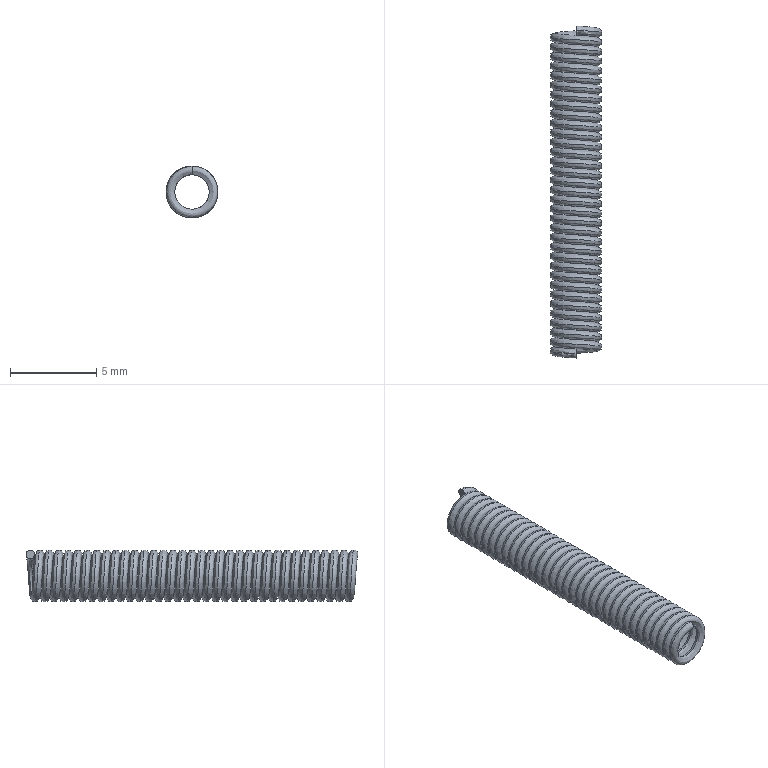Part | SolidWorks | features Helix 1, Sweep 1 | 1 solid | 4 faces | box 3 x 19.2 x 3 mm | volume 52.414 mm3 | spline 2 | plane 2